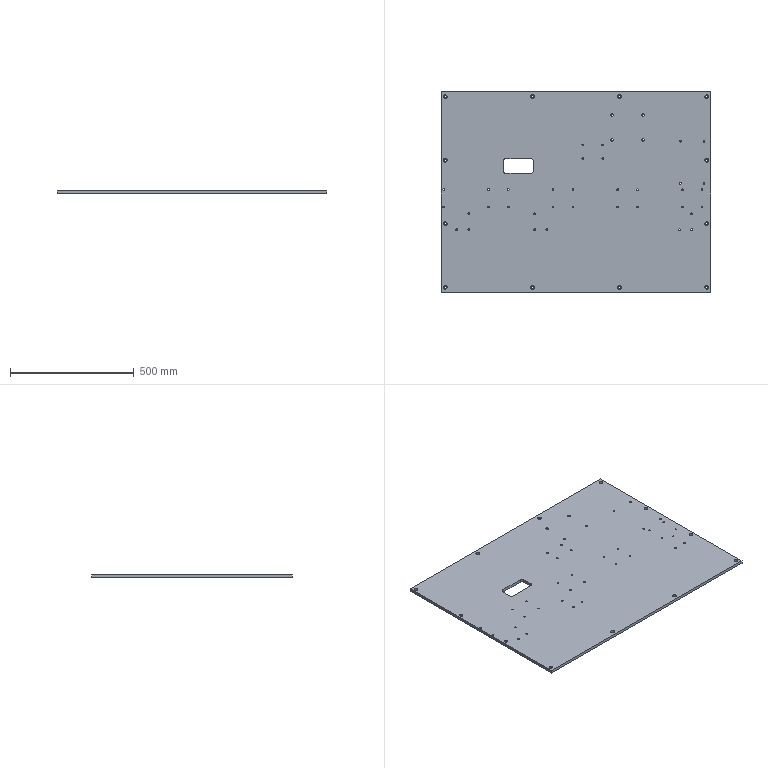Part | STEP file | X77-03006 | 1 solid | 152 faces | box 1087 x 810 x 12 mm | volume 10436415 mm3 | cylinder 130 | plane 22 | commonest cylinder face diameters 6.8 x70 9 x24 15 x24 10.2 x8 20 x4